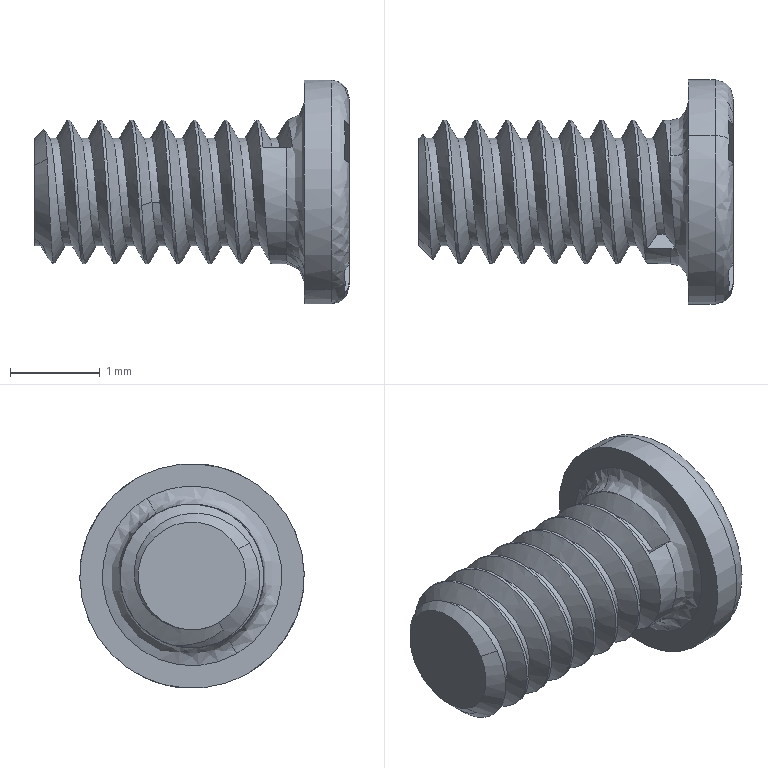Part | SolidWorks | features BaseBody 1 | 1 solid | 59 faces | box 3.5 x 2.5 x 2.5 mm | volume 6.379 mm3 | spline 59